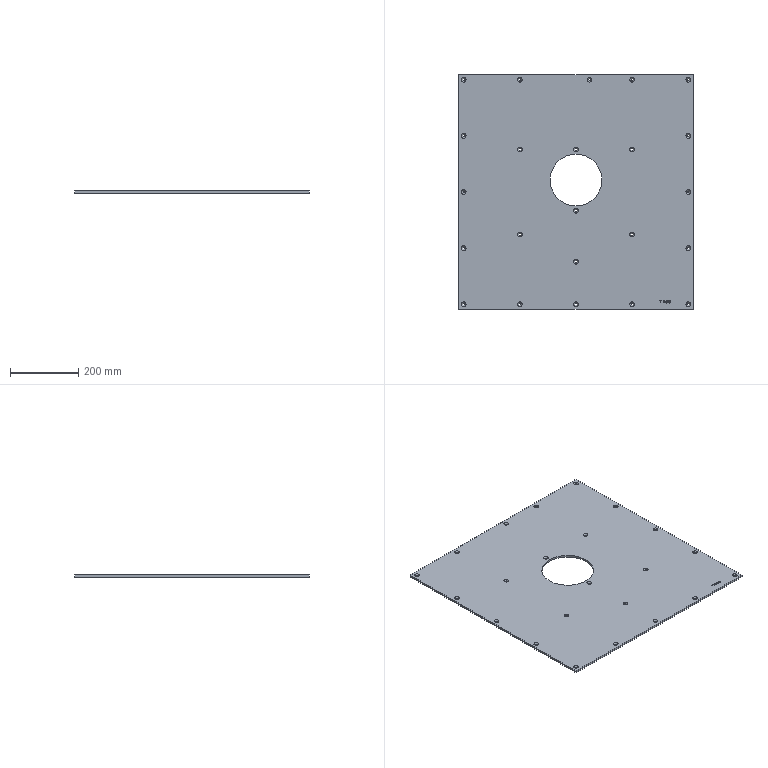Part | Creo | 1 solid | 173 faces | box 690 x 690 x 6 mm | volume 2738784 mm3 | other 54 | cylinder 48 | cone 46 | plane 25 | commonest cylinder face diameters 7 x46 152 x2